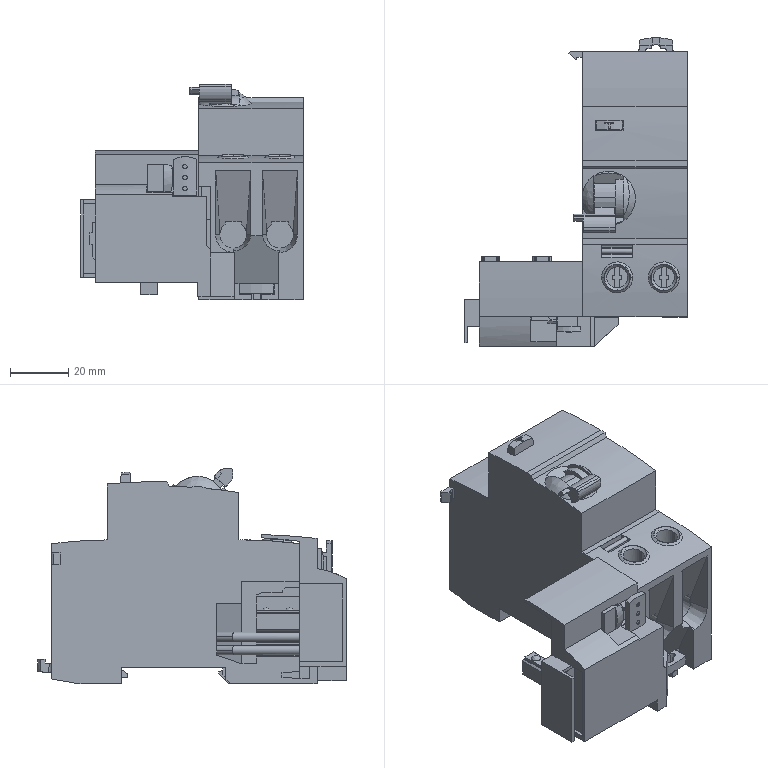Part | STEP file | Residual current device Vigi-iC65-ELE-2P-40A-30mA-A | 16 solids | 725 faces | box 76.2 x 105.618 x 73.908 mm | volume 172404 mm3 | plane 593 | cylinder 110 | spline 18 | cone 4 | commonest cylinder face diameters 3.2 x13 7.2 x8 8.4 x8 2 x7 1.466 x6 9.2 x6